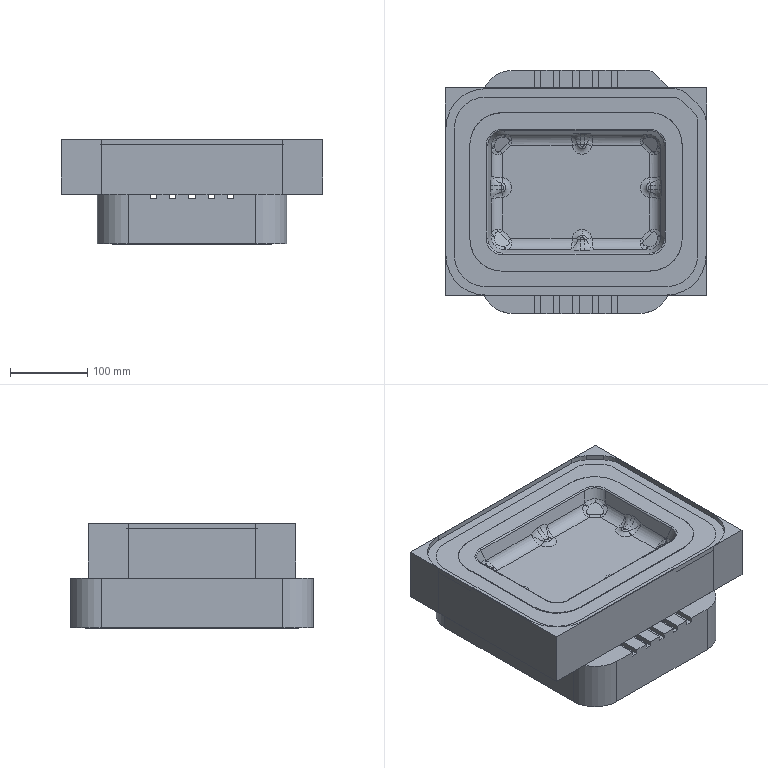NC program | NX | posted with a generic post | part box 339.125 x 315.125 x 135.5 mm
Lines 1 to 1308 of 120728:
N10 G17 G21 G94 G90
(B1 , TOOL : D16R0.8)
N12 T00 M6
N14 G53
N16 G17 G0 G90 X-27.429 Y125.5 S7000 M3 M8
N18 G43 Z220.5 H0
N20 Z71.5
N22 G94 G1 X0. Z70.063 F4500.
N24 X126.349
N26 G2 X138.946 Y120.282 R17.815
N28 G1 X155.159 Y104.069
N30 G2 X160.377 Y91.472 R17.815
N32 G1 Y-82.685
N34 G2 X117.563 Y-125.5 R42.815
N36 G1 X-117.563
N38 G2 X-160.377 Y-82.685 R42.815
N40 G1 Y82.685
N42 G2 X-117.563 Y125.5 R42.815
N44 G1 X0.
N46 Y115.42
N48 X126.349
N50 G2 X131.818 Y113.154 R7.735
N52 G1 X148.032 Y96.941
N54 G2 X150.297 Y91.472 R7.735
N56 G1 Y-82.685
N58 G2 X117.563 Y-115.42 R32.735
N60 G1 X-117.563
N62 G2 X-150.297 Y-82.685 R32.735
N64 G1 Y82.685
N66 G2 X-117.563 Y115.42 R32.735
N68 G1 X0.
N70 Y105.34
N72 X125.378
N74 X140.217 Y90.5
N76 Y-82.685
N78 G2 X117.563 Y-105.34 R22.655
N80 G1 X-117.563
N82 G2 X-140.217 Y-82.685 R22.655
N84 G1 Y82.685
N86 G2 X-117.563 Y105.34 R22.655
N88 G1 X0.
N90 Y95.26
N92 X121.203
N94 X130.137 Y86.325
N96 Y-82.685
N98 G2 X117.563 Y-95.26 R12.575
N100 G1 X-117.563
N102 G2 X-130.137 Y-82.685 R12.575
N104 G1 Y82.685
N106 G2 X-117.563 Y95.26 R12.575
N108 G1 X0.
N110 Y85.18
N112 X117.027
N114 X120.057 Y82.15
N116 Y-82.685
N118 G2 X117.563 Y-85.18 R2.495
N120 G1 X-117.563
N122 G2 X-120.057 Y-82.685 R2.495
N124 G1 Y82.685
N126 G2 X-117.563 Y85.18 R2.495
N128 G1 X0.
N130 Y75.1
N132 X109.977
N134 Y-75.1
N136 X-109.977
N138 Y75.1
N140 X0.
N142 Y65.02
N144 X99.897
N146 Y-65.02
N148 X-99.897
N150 Y65.02
N152 X0.
N154 Y54.94
N156 X89.817
N158 Y-54.94
N160 X-89.817
N162 Y54.94
N164 X0.
N166 Y44.86
N168 X79.737
N170 Y-44.86
N172 X-79.737
N174 Y44.86
N176 X0.
N178 Y34.78
N180 X69.657
N182 Y-34.78
N184 X-69.657
N186 Y34.78
N188 X0.
N190 Y24.7
N192 X59.577
N194 Y-24.7
N196 X-59.577
N198 Y24.7
N200 X0.
N202 Y14.62
N204 X49.497
N206 Y-14.62
N208 X-49.497
N210 Y14.62
N212 X0.
N214 Y4.54
N216 X39.417
N218 Y-4.54
N220 X-39.417
N222 Y4.54
N224 X0.
N226 G3 X3.2 Y7.74 R3.2
N228 G1 Z71.063
N230 G0 Z73.5
N232 X-27.429 Y125.435
N234 Z71.063
N236 G1 X0. Z69.625
N238 X126.349
N240 G2 X138.9 Y120.236 R17.75
N242 G1 X155.114 Y104.023
N244 G2 X160.313 Y91.472 R17.75
N246 G1 Y-82.685
N248 G2 X117.563 Y-125.435 R42.75
N250 G1 X-117.563
N252 G2 X-160.313 Y-82.685 R42.75
N254 G1 Y82.685
N256 G2 X-117.563 Y125.435 R42.75
N258 G1 X0.
N260 Y115.355
N262 X126.349
N264 G2 X131.773 Y113.109 R7.67
N266 G1 X147.986 Y96.895
N268 G2 X150.233 Y91.472 R7.67
N270 G1 Y-82.685
N272 G2 X117.563 Y-115.355 R32.67
N274 G1 X-117.563
N276 G2 X-150.233 Y-82.685 R32.67
N278 G1 Y82.685
N280 G2 X-117.563 Y115.355 R32.67
N282 G1 X0.
N284 Y105.275
N286 X125.351
N288 X140.153 Y90.474
N290 Y-82.686
N292 G2 X117.563 Y-105.275 R22.59
N294 G1 X-117.563
N296 G2 X-140.153 Y-82.685 R22.59
N298 G1 Y82.685
N300 G2 X-117.563 Y105.275 R22.59
N302 G1 X0.
N304 Y95.195
N306 X121.176
N308 X130.073 Y86.298
N310 Y-82.687
N312 G2 X117.563 Y-95.195 R12.51
N314 G1 X-117.563
N316 G2 X-130.073 Y-82.685 R12.51
N318 G1 Y82.685
N320 G2 X-117.563 Y95.195 R12.51
N322 G1 X0.
N324 Y85.115
N326 X117.
N328 X119.993 Y82.123
N330 Y-82.686
N332 G2 X117.563 Y-85.115 R2.43
N334 G1 X-117.563
N336 G2 X-119.993 Y-82.685 R2.43
N338 G1 Y82.685
N340 G2 X-117.563 Y85.115 R2.43
N342 G1 X0.
N344 Y75.035
N346 X109.913
N348 Y-75.035
N350 X-109.913
N352 Y75.035
N354 X0.
N356 Y64.955
N358 X99.833
N360 Y-64.955
N362 X-99.833
N364 Y64.955
N366 X0.
N368 Y54.875
N370 X89.753
N372 Y-54.875
N374 X-89.753
N376 Y54.875
N378 X0.
N380 Y44.795
N382 X79.673
N384 Y-44.795
N386 X-79.673
N388 Y44.795
N390 X0.
N392 Y34.715
N394 X69.593
N396 Y-34.715
N398 X-69.593
N400 Y34.715
N402 X0.
N404 Y24.635
N406 X59.513
N408 Y-24.635
N410 X-59.513
N412 Y24.635
N414 X0.
N416 Y14.555
N418 X49.433
N420 Y-14.555
N422 X-49.433
N424 Y14.555
N426 X0.
N428 Y4.475
N430 X39.353
N432 Y-4.475
N434 X-39.353
N436 Y4.475
N438 X0.
N440 G3 X3.2 Y7.675 R3.2
N442 G1 Z70.625
N444 G0 Z73.063
N446 X-27.429 Y125.435
N448 Z70.625
N450 G1 X0. Z69.188
N452 X126.349
N454 G2 X138.9 Y120.236 R17.75
N456 G1 X155.114 Y104.023
N458 G2 X160.313 Y91.472 R17.75
N460 G1 Y-82.685
N462 G2 X117.563 Y-125.435 R42.75
N464 G1 X-117.563
N466 G2 X-160.313 Y-82.685 R42.75
N468 G1 Y82.685
N470 G2 X-117.563 Y125.435 R42.75
N472 G1 X0.
N474 Y115.355
N476 X126.349
N478 G2 X131.773 Y113.109 R7.67
N480 G1 X147.986 Y96.895
N482 G2 X150.233 Y91.472 R7.67
N484 G1 Y-82.685
N486 G2 X117.563 Y-115.355 R32.67
N488 G1 X-117.563
N490 G2 X-150.233 Y-82.685 R32.67
N492 G1 Y82.685
N494 G2 X-117.563 Y115.355 R32.67
N496 G1 X0.
N498 Y105.275
N500 X125.351
N502 X140.153 Y90.474
N504 Y-82.686
N506 G2 X117.563 Y-105.275 R22.59
N508 G1 X-117.563
N510 G2 X-140.153 Y-82.685 R22.59
N512 G1 Y82.685
N514 G2 X-117.563 Y105.275 R22.59
N516 G1 X0.
N518 Y95.195
N520 X121.176
N522 X130.073 Y86.298
N524 Y-82.687
N526 G2 X117.563 Y-95.195 R12.51
N528 G1 X-117.563
N530 G2 X-130.073 Y-82.685 R12.51
N532 G1 Y82.685
N534 G2 X-117.563 Y95.195 R12.51
N536 G1 X0.
N538 Y85.115
N540 X117.
N542 X119.993 Y82.123
N544 Y-82.686
N546 G2 X117.563 Y-85.115 R2.43
N548 G1 X-117.563
N550 G2 X-119.993 Y-82.685 R2.43
N552 G1 Y82.685
N554 G2 X-117.563 Y85.115 R2.43
N556 G1 X0.
N558 Y75.035
N560 X109.913
N562 Y-75.035
N564 X-109.913
N566 Y75.035
N568 X0.
N570 Y64.955
N572 X99.833
N574 Y-64.955
N576 X-99.833
N578 Y64.955
N580 X0.
N582 Y54.875
N584 X89.753
N586 Y-54.875
N588 X-89.753
N590 Y54.875
N592 X0.
N594 Y44.795
N596 X79.673
N598 Y-44.795
N600 X-79.673
N602 Y44.795
N604 X0.
N606 Y34.715
N608 X69.593
N610 Y-34.715
N612 X-69.593
N614 Y34.715
N616 X0.
N618 Y24.635
N620 X59.513
N622 Y-24.635
N624 X-59.513
N626 Y24.635
N628 X0.
N630 Y14.555
N632 X49.433
N634 Y-14.555
N636 X-49.433
N638 Y14.555
N640 X0.
N642 Y4.475
N644 X39.353
N646 Y-4.475
N648 X-39.353
N650 Y4.475
N652 X0.
N654 G3 X3.2 Y7.675 R3.2
N656 G1 Z70.188
N658 G0 Z72.625
N660 X-27.429 Y125.435
N662 Z70.188
N664 G1 X0. Z68.75
N666 X126.349
N668 G2 X138.9 Y120.236 R17.75
N670 G1 X155.114 Y104.023
N672 G2 X160.313 Y91.472 R17.75
N674 G1 Y-82.685
N676 G2 X117.563 Y-125.435 R42.75
N678 G1 X-117.563
N680 G2 X-160.313 Y-82.685 R42.75
N682 G1 Y82.685
N684 G2 X-117.563 Y125.435 R42.75
N686 G1 X0.
N688 Y115.355
N690 X126.349
N692 G2 X131.773 Y113.109 R7.67
N694 G1 X147.986 Y96.895
N696 G2 X150.233 Y91.472 R7.67
N698 G1 Y-82.685
N700 G2 X117.563 Y-115.355 R32.67
N702 G1 X-117.563
N704 G2 X-150.233 Y-82.685 R32.67
N706 G1 Y82.685
N708 G2 X-117.563 Y115.355 R32.67
N710 G1 X0.
N712 Y105.275
N714 X125.351
N716 X140.153 Y90.474
N718 Y-82.686
N720 G2 X117.563 Y-105.275 R22.59
N722 G1 X-117.563
N724 G2 X-140.153 Y-82.685 R22.59
N726 G1 Y82.685
N728 G2 X-117.563 Y105.275 R22.59
N730 G1 X0.
N732 Y95.195
N734 X121.176
N736 X130.073 Y86.298
N738 Y-82.687
N740 G2 X117.563 Y-95.195 R12.51
N742 G1 X-117.563
N744 G2 X-130.073 Y-82.685 R12.51
N746 G1 Y82.685
N748 G2 X-117.563 Y95.195 R12.51
N750 G1 X0.
N752 Y85.115
N754 X117.
N756 X119.993 Y82.123
N758 Y-82.686
N760 G2 X117.563 Y-85.115 R2.43
N762 G1 X-117.563
N764 G2 X-119.993 Y-82.685 R2.43
N766 G1 Y82.685
N768 G2 X-117.563 Y85.115 R2.43
N770 G1 X0.
N772 Y75.035
N774 X109.913
N776 Y-75.035
N778 X-109.913
N780 Y75.035
N782 X0.
N784 Y64.955
N786 X99.833
N788 Y-64.955
N790 X-99.833
N792 Y64.955
N794 X0.
N796 Y54.875
N798 X89.753
N800 Y-54.875
N802 X-89.753
N804 Y54.875
N806 X0.
N808 Y44.795
N810 X79.673
N812 Y-44.795
N814 X-79.673
N816 Y44.795
N818 X0.
N820 Y34.715
N822 X69.593
N824 Y-34.715
N826 X-69.593
N828 Y34.715
N830 X0.
N832 Y24.635
N834 X59.513
N836 Y-24.635
N838 X-59.513
N840 Y24.635
N842 X0.
N844 Y14.555
N846 X49.433
N848 Y-14.555
N850 X-49.433
N852 Y14.555
N854 X0.
N856 Y4.475
N858 X39.353
N860 Y-4.475
N862 X-39.353
N864 Y4.475
N866 X0.
N868 G3 X3.2 Y7.675 R3.2
N870 G1 Z69.75
N872 G0 Z72.188
N874 X-27.429 Y125.435
N876 Z69.75
N878 G1 X0. Z68.313
N880 X126.349
N882 G2 X138.9 Y120.236 R17.75
N884 G1 X155.114 Y104.023
N886 G2 X160.313 Y91.472 R17.75
N888 G1 Y-82.685
N890 G2 X117.563 Y-125.435 R42.75
N892 G1 X-117.563
N894 G2 X-160.313 Y-82.685 R42.75
N896 G1 Y82.685
N898 G2 X-117.563 Y125.435 R42.75
N900 G1 X0.
N902 Y115.355
N904 X126.349
N906 G2 X131.773 Y113.109 R7.67
N908 G1 X147.986 Y96.895
N910 G2 X150.233 Y91.472 R7.67
N912 G1 Y-82.685
N914 G2 X117.563 Y-115.355 R32.67
N916 G1 X-117.563
N918 G2 X-150.233 Y-82.685 R32.67
N920 G1 Y82.685
N922 G2 X-117.563 Y115.355 R32.67
N924 G1 X0.
N926 Y105.275
N928 X125.351
N930 X140.153 Y90.474
N932 Y-82.686
N934 G2 X117.563 Y-105.275 R22.59
N936 G1 X-117.563
N938 G2 X-140.153 Y-82.685 R22.59
N940 G1 Y82.685
N942 G2 X-117.563 Y105.275 R22.59
N944 G1 X0.
N946 Y95.195
N948 X121.176
N950 X130.073 Y86.298
N952 Y-82.687
N954 G2 X117.563 Y-95.195 R12.51
N956 G1 X-117.563
N958 G2 X-130.073 Y-82.685 R12.51
N960 G1 Y82.685
N962 G2 X-117.563 Y95.195 R12.51
N964 G1 X0.
N966 Y85.115
N968 X117.
N970 X119.993 Y82.123
N972 Y-82.686
N974 G2 X117.563 Y-85.115 R2.43
N976 G1 X-117.563
N978 G2 X-119.993 Y-82.685 R2.43
N980 G1 Y82.685
N982 G2 X-117.563 Y85.115 R2.43
N984 G1 X0.
N986 Y75.035
N988 X109.913
N990 Y-75.035
N992 X-109.913
N994 Y75.035
N996 X0.
N998 Y64.955
N1000 X99.833
N1002 Y-64.955
N1004 X-99.833
N1006 Y64.955
N1008 X0.
N1010 Y54.875
N1012 X89.753
N1014 Y-54.875
N1016 X-89.753
N1018 Y54.875
N1020 X0.
N1022 Y44.795
N1024 X79.673
N1026 Y-44.795
N1028 X-79.673
N1030 Y44.795
N1032 X0.
N1034 Y34.715
N1036 X69.593
N1038 Y-34.715
N1040 X-69.593
N1042 Y34.715
N1044 X0.
N1046 Y24.635
N1048 X59.513
N1050 Y-24.635
N1052 X-59.513
N1054 Y24.635
N1056 X0.
N1058 Y14.555
N1060 X49.433
N1062 Y-14.555
N1064 X-49.433
N1066 Y14.555
N1068 X0.
N1070 Y4.475
N1072 X39.353
N1074 Y-4.475
N1076 X-39.353
N1078 Y4.475
N1080 X0.
N1082 G3 X3.2 Y7.675 R3.2
N1084 G1 Z69.313
N1086 G0 Z71.75
N1088 X-27.429 Y125.435
N1090 Z69.313
N1092 G1 X0. Z67.875
N1094 X126.349
N1096 G2 X138.9 Y120.236 R17.75
N1098 G1 X155.114 Y104.023
N1100 G2 X160.313 Y91.472 R17.75
N1102 G1 Y-82.685
N1104 G2 X117.563 Y-125.435 R42.75
N1106 G1 X-117.563
N1108 G2 X-160.313 Y-82.685 R42.75
N1110 G1 Y82.685
N1112 G2 X-117.563 Y125.435 R42.75
N1114 G1 X0.
N1116 Y115.355
N1118 X126.349
N1120 G2 X131.773 Y113.109 R7.67
N1122 G1 X147.986 Y96.895
N1124 G2 X150.233 Y91.472 R7.67
N1126 G1 Y-82.685
N1128 G2 X117.563 Y-115.355 R32.67
N1130 G1 X-117.563
N1132 G2 X-150.233 Y-82.685 R32.67
N1134 G1 Y82.685
N1136 G2 X-117.563 Y115.355 R32.67
N1138 G1 X0.
N1140 Y105.275
N1142 X125.351
N1144 X140.153 Y90.474
N1146 Y-82.686
N1148 G2 X117.563 Y-105.275 R22.59
N1150 G1 X-117.563
N1152 G2 X-140.153 Y-82.685 R22.59
N1154 G1 Y82.685
N1156 G2 X-117.563 Y105.275 R22.59
N1158 G1 X0.
N1160 Y95.195
N1162 X121.176
N1164 X130.073 Y86.298
N1166 Y-82.687
N1168 G2 X117.563 Y-95.195 R12.51
N1170 G1 X-117.563
N1172 G2 X-130.073 Y-82.685 R12.51
N1174 G1 Y82.685
N1176 G2 X-117.563 Y95.195 R12.51
N1178 G1 X0.
N1180 Y85.115
N1182 X117.
N1184 X119.993 Y82.123
N1186 Y-82.686
N1188 G2 X117.563 Y-85.115 R2.43
N1190 G1 X-117.563
N1192 G2 X-119.993 Y-82.685 R2.43
N1194 G1 Y82.685
N1196 G2 X-117.563 Y85.115 R2.43
N1198 G1 X0.
N1200 Y75.035
N1202 X109.913
N1204 Y-75.035
N1206 X-109.913
N1208 Y75.035
N1210 X0.
N1212 Y64.955
N1214 X99.833
N1216 Y-64.955
N1218 X-99.833
N1220 Y64.955
N1222 X0.
N1224 Y54.875
N1226 X89.753
N1228 Y-54.875
N1230 X-89.753
N1232 Y54.875
N1234 X0.
N1236 Y44.795
N1238 X79.673
N1240 Y-44.795
N1242 X-79.673
N1244 Y44.795
N1246 X0.
N1248 Y34.715
N1250 X69.593
N1252 Y-34.715
N1254 X-69.593
N1256 Y34.715
N1258 X0.
N1260 Y24.635
N1262 X59.513
N1264 Y-24.635
N1266 X-59.513
N1268 Y24.635
N1270 X0.
N1272 Y14.555
N1274 X49.433
N1276 Y-14.555
N1278 X-49.433
N1280 Y14.555
N1282 X0.
N1284 Y4.475
N1286 X39.353
N1288 Y-4.475
N1290 X-39.353
N1292 Y4.475
N1294 X0.
N1296 G3 X3.2 Y7.675 R3.2
N1298 G1 Z68.875
N1300 G0 Z71.313
N1302 X-27.429 Y125.435
N1304 Z68.875
N1306 G1 X0. Z67.438
N1308 X126.349
N1310 G2 X138.9 Y120.236 R17.75
N1312 G1 X155.114 Y104.023
N1314 G2 X160.313 Y91.472 R17.75
N1316 G1 Y-82.685
N1318 G2 X117.563 Y-125.435 R42.75
N1320 G1 X-117.563
N1322 G2 X-160.313 Y-82.685 R42.75
N1324 G1 Y82.685
N1326 G2 X-117.563 Y125.435 R42.75
N1328 G1 X0.
N1330 Y115.355
N1332 X126.349
N1334 G2 X131.773 Y113.109 R7.67
N1336 G1 X147.986 Y96.895
N1338 G2 X150.233 Y91.472 R7.67
N1340 G1 Y-82.685
N1342 G2 X117.563 Y-115.355 R32.67
N1344 G1 X-117.563
N1346 G2 X-150.233 Y-82.685 R32.67
N1348 G1 Y82.685
N1350 G2 X-117.563 Y115.355 R32.67
N1352 G1 X0.
N1354 Y105.275
N1356 X125.351
N1358 X140.153 Y90.474
N1360 Y-82.686
N1362 G2 X117.563 Y-105.275 R22.59
N1364 G1 X-117.563
N1366 G2 X-140.153 Y-82.685 R22.59
N1368 G1 Y82.685
N1370 G2 X-117.563 Y105.275 R22.59
N1372 G1 X0.
N1374 Y95.195
N1376 X121.176
N1378 X130.073 Y86.298
N1380 Y-82.687
N1382 G2 X117.563 Y-95.195 R12.51
N1384 G1 X-117.563
N1386 G2 X-130.073 Y-82.685 R12.51
N1388 G1 Y82.685
N1390 G2 X-117.563 Y95.195 R12.51
N1392 G1 X0.
N1394 Y85.115
N1396 X117.
N1398 X119.993 Y82.123
N1400 Y-82.686
N1402 G2 X117.563 Y-85.115 R2.43
N1404 G1 X-117.563
N1406 G2 X-119.993 Y-82.685 R2.43
N1408 G1 Y82.685
N1410 G2 X-117.563 Y85.115 R2.43
N1412 G1 X0.
N1414 Y75.035
N1416 X109.913
N1418 Y-75.035
N1420 X-109.913
N1422 Y75.035
N1424 X0.
N1426 Y64.955
N1428 X99.833
N1430 Y-64.955
N1432 X-99.833
N1434 Y64.955
N1436 X0.
N1438 Y54.875
N1440 X89.753
N1442 Y-54.875
N1444 X-89.753
N1446 Y54.875
N1448 X0.
N1450 Y44.795
N1452 X79.673
N1454 Y-44.795
N1456 X-79.673
N1458 Y44.795
N1460 X0.
N1462 Y34.715
N1464 X69.593
N1466 Y-34.715
N1468 X-69.593
N1470 Y34.715
N1472 X0.
N1474 Y24.635
N1476 X59.513
N1478 Y-24.635
N1480 X-59.513
N1482 Y24.635
N1484 X0.
N1486 Y14.555
N1488 X49.433
N1490 Y-14.555
N1492 X-49.433
N1494 Y14.555
N1496 X0.
N1498 Y4.475
N1500 X39.353
N1502 Y-4.475
N1504 X-39.353
N1506 Y4.475
N1508 X0.
N1510 G3 X3.2 Y7.675 R3.2
N1512 G1 Z68.438
N1514 G0 Z70.875
N1516 X-27.429 Y125.435
N1518 Z68.438
N1520 G1 X0. Z67.
N1522 X126.349
N1524 G2 X138.9 Y120.236 R17.75
N1526 G1 X155.114 Y104.023
N1528 G2 X160.313 Y91.472 R17.75
N1530 G1 Y-82.685
N1532 G2 X117.563 Y-125.435 R42.75
N1534 G1 X-117.563
N1536 G2 X-160.313 Y-82.685 R42.75
N1538 G1 Y82.685
N1540 G2 X-117.563 Y125.435 R42.75
N1542 G1 X0.
N1544 Y115.355
N1546 X126.349
N1548 G2 X131.773 Y113.109 R7.67
N1550 G1 X147.986 Y96.895
N1552 G2 X150.233 Y91.472 R7.67
N1554 G1 Y-82.685
N1556 G2 X117.563 Y-115.355 R32.67
N1558 G1 X-117.563
N1560 G2 X-150.233 Y-82.685 R32.67
N1562 G1 Y82.685
N1564 G2 X-117.563 Y115.355 R32.67
N1566 G1 X0.
N1568 Y105.275
N1570 X125.351
N1572 X140.153 Y90.474
N1574 Y-82.686
N1576 G2 X117.563 Y-105.275 R22.59
N1578 G1 X-117.563
N1580 G2 X-140.153 Y-82.685 R22.59
N1582 G1 Y82.685
N1584 G2 X-117.563 Y105.275 R22.59
N1586 G1 X0.
N1588 Y95.195
N1590 X121.176
N1592 X130.073 Y86.298
N1594 Y-82.687
N1596 G2 X117.563 Y-95.195 R12.51
N1598 G1 X-117.563
N1600 G2 X-130.073 Y-82.685 R12.51
N1602 G1 Y82.685
N1604 G2 X-117.563 Y95.195 R12.51
N1606 G1 X0.
N1608 Y85.115
N1610 X117.
N1612 X119.993 Y82.123
N1614 Y-82.686
N1616 G2 X117.563 Y-85.115 R2.43
N1618 G1 X-117.563
N1620 G2 X-119.993 Y-82.685 R2.43
N1622 G1 Y82.685
N1624 G2 X-117.563 Y85.115 R2.43
N1626 G1 X0.
N1628 Y75.035
N1630 X109.913
N1632 Y-75.035
N1634 X-109.913
N1636 Y75.035
N1638 X0.
N1640 Y64.955
N1642 X99.833
N1644 Y-64.955
N1646 X-99.833
N1648 Y64.955
N1650 X0.
N1652 Y54.875
N1654 X89.753
N1656 Y-54.875
N1658 X-89.753
N1660 Y54.875
N1662 X0.
N1664 Y44.795
N1666 X79.673
N1668 Y-44.795
N1670 X-79.673
N1672 Y44.795
N1674 X0.
N1676 Y34.715
N1678 X69.593
N1680 Y-34.715
N1682 X-69.593
N1684 Y34.715
N1686 X0.
N1688 Y24.635
N1690 X59.513
N1692 Y-24.635
N1694 X-59.513
N1696 Y24.635
N1698 X0.
N1700 Y14.555
N1702 X49.433
N1704 Y-14.555
N1706 X-49.433
N1708 Y14.555
N1710 X0.
N1712 Y4.475
N1714 X39.353
N1716 Y-4.475
N1718 X-39.353
N1720 Y4.475
N1722 X0.
N1724 G3 X3.2 Y7.675 R3.2
N1726 G1 Z68.
N1728 G0 Z70.438
N1730 X-27.429 Y125.435
N1732 Z68.
N1734 G1 X0. Z66.563
N1736 X126.349
N1738 G2 X138.9 Y120.236 R17.75
N1740 G1 X155.114 Y104.023
N1742 G2 X160.313 Y91.472 R17.75
N1744 G1 Y-82.685
N1746 G2 X117.563 Y-125.435 R42.75
N1748 G1 X-117.563
N1750 G2 X-160.313 Y-82.685 R42.75
N1752 G1 Y82.685
N1754 G2 X-117.563 Y125.435 R42.75
N1756 G1 X0.
N1758 Y115.355
N1760 X126.349
N1762 G2 X131.773 Y113.109 R7.67
N1764 G1 X147.986 Y96.895
N1766 G2 X150.233 Y91.472 R7.67
N1768 G1 Y-82.685
N1770 G2 X117.563 Y-115.355 R32.67
N1772 G1 X-117.563
N1774 G2 X-150.233 Y-82.685 R32.67
N1776 G1 Y82.685
N1778 G2 X-117.563 Y115.355 R32.67
N1780 G1 X0.
N1782 Y105.275
N1784 X125.351
N1786 X140.153 Y90.474
N1788 Y-82.686
N1790 G2 X117.563 Y-105.275 R22.59
N1792 G1 X-117.563
N1794 G2 X-140.153 Y-82.685 R22.59
N1796 G1 Y82.685
N1798 G2 X-117.563 Y105.275 R22.59
N1800 G1 X0.
N1802 Y95.195
N1804 X121.176
N1806 X130.073 Y86.298
N1808 Y-82.687
N1810 G2 X117.563 Y-95.195 R12.51
N1812 G1 X-117.563
N1814 G2 X-130.073 Y-82.685 R12.51
N1816 G1 Y82.685
N1818 G2 X-117.563 Y95.195 R12.51
N1820 G1 X0.
N1822 Y85.115
N1824 X117.
N1826 X119.993 Y82.123
N1828 Y-82.686
N1830 G2 X117.563 Y-85.115 R2.43
N1832 G1 X-117.563
N1834 G2 X-119.993 Y-82.685 R2.43
N1836 G1 Y82.685
N1838 G2 X-117.563 Y85.115 R2.43
N1840 G1 X0.
N1842 Y75.035
N1844 X109.913
N1846 Y-75.035
N1848 X-109.913
N1850 Y75.035
N1852 X0.
N1854 Y64.955
N1856 X99.833
N1858 Y-64.955
N1860 X-99.833
N1862 Y64.955
N1864 X0.
N1866 Y54.875
N1868 X89.753
N1870 Y-54.875
N1872 X-89.753
N1874 Y54.875
N1876 X0.
N1878 Y44.795
N1880 X79.673
N1882 Y-44.795
N1884 X-79.673
N1886 Y44.795
N1888 X0.
N1890 Y34.715
N1892 X69.593
N1894 Y-34.715
N1896 X-69.593
N1898 Y34.715
N1900 X0.
N1902 Y24.635
N1904 X59.513
N1906 Y-24.635
N1908 X-59.513
N1910 Y24.635
N1912 X0.
N1914 Y14.555
N1916 X49.433
N1918 Y-14.555
N1920 X-49.433
N1922 Y14.555
N1924 X0.
N1926 Y4.475
N1928 X39.353
N1930 Y-4.475
N1932 X-39.353
N1934 Y4.475
N1936 X0.
N1938 G3 X3.2 Y7.675 R3.2
N1940 G1 Z67.563
N1942 G0 Z70.
N1944 X-27.429 Y125.435
N1946 Z67.563
N1948 G1 X0. Z66.125
N1950 X126.349
N1952 G2 X138.9 Y120.236 R17.75
N1954 G1 X155.114 Y104.023
N1956 G2 X160.313 Y91.472 R17.75
N1958 G1 Y-82.685
N1960 G2 X117.563 Y-125.435 R42.75
N1962 G1 X-117.563
N1964 G2 X-160.313 Y-82.685 R42.75
N1966 G1 Y82.685
N1968 G2 X-117.563 Y125.435 R42.75
N1970 G1 X0.
N1972 Y115.355
N1974 X126.349
N1976 G2 X131.773 Y113.109 R7.67
N1978 G1 X147.986 Y96.895
N1980 G2 X150.233 Y91.472 R7.67
N1982 G1 Y-82.685
N1984 G2 X117.563 Y-115.355 R32.67
N1986 G1 X-117.563
N1988 G2 X-150.233 Y-82.685 R32.67
N1990 G1 Y82.685
N1992 G2 X-117.563 Y115.355 R32.67
N1994 G1 X0.
N1996 Y105.275
N1998 X125.351
N2000 X140.153 Y90.474
N2002 Y-82.686
N2004 G2 X117.563 Y-105.275 R22.59
N2006 G1 X-117.563
N2008 G2 X-140.153 Y-82.685 R22.59
N2010 G1 Y82.685
N2012 G2 X-117.563 Y105.275 R22.59
N2014 G1 X0.
N2016 Y95.195
N2018 X121.176
N2020 X130.073 Y86.298
N2022 Y-82.687
N2024 G2 X117.563 Y-95.195 R12.51
N2026 G1 X-117.563
N2028 G2 X-130.073 Y-82.685 R12.51
N2030 G1 Y82.685
N2032 G2 X-117.563 Y95.195 R12.51
N2034 G1 X0.
N2036 Y85.115
N2038 X117.
N2040 X119.993 Y82.123
N2042 Y-82.686
N2044 G2 X117.563 Y-85.115 R2.43
N2046 G1 X-117.563
N2048 G2 X-119.993 Y-82.685 R2.43
N2050 G1 Y82.685
N2052 G2 X-117.563 Y85.115 R2.43
N2054 G1 X0.
N2056 Y75.035
N2058 X109.913
N2060 Y-75.035
N2062 X-109.913
N2064 Y75.035
N2066 X0.
N2068 Y64.955
N2070 X99.833
N2072 Y-64.955
N2074 X-99.833
N2076 Y64.955
N2078 X0.
N2080 Y54.875
N2082 X89.753
N2084 Y-54.875
N2086 X-89.753
N2088 Y54.875
N2090 X0.
N2092 Y44.795
N2094 X79.673
N2096 Y-44.795
N2098 X-79.673
N2100 Y44.795
N2102 X0.
N2104 Y34.715
N2106 X69.593
N2108 Y-34.715
N2110 X-69.593
N2112 Y34.715
N2114 X0.
N2116 Y24.635
N2118 X59.513
N2120 Y-24.635
N2122 X-59.513
N2124 Y24.635
N2126 X0.
N2128 Y14.555
N2130 X49.433
N2132 Y-14.555
N2134 X-49.433
N2136 Y14.555
N2138 X0.
N2140 Y4.475
N2142 X39.353
N2144 Y-4.475
N2146 X-39.353
N2148 Y4.475
N2150 X0.
N2152 G3 X3.2 Y7.675 R3.2
N2154 G1 Z67.125
N2156 G0 Z69.563
N2158 X-27.429 Y125.435
N2160 Z67.125
N2162 G1 X0. Z65.688
N2164 X126.349
N2166 G2 X138.9 Y120.236 R17.75
N2168 G1 X155.114 Y104.023
N2170 G2 X160.313 Y91.472 R17.75
N2172 G1 Y-82.685
N2174 G2 X117.563 Y-125.435 R42.75
N2176 G1 X-117.563
N2178 G2 X-160.313 Y-82.685 R42.75
N2180 G1 Y82.685
N2182 G2 X-117.563 Y125.435 R42.75
N2184 G1 X0.
N2186 Y115.355
N2188 X126.349
N2190 G2 X131.773 Y113.109 R7.67
N2192 G1 X147.986 Y96.895
N2194 G2 X150.233 Y91.472 R7.67
N2196 G1 Y-82.685
N2198 G2 X117.563 Y-115.355 R32.67
N2200 G1 X-117.563
N2202 G2 X-150.233 Y-82.685 R32.67
N2204 G1 Y82.685
N2206 G2 X-117.563 Y115.355 R32.67
N2208 G1 X0.
N2210 Y105.275
N2212 X125.351
N2214 X140.153 Y90.474
N2216 Y-82.686
N2218 G2 X117.563 Y-105.275 R22.59
N2220 G1 X-117.563
N2222 G2 X-140.153 Y-82.685 R22.59
N2224 G1 Y82.685
N2226 G2 X-117.563 Y105.275 R22.59
N2228 G1 X0.
N2230 Y95.195
N2232 X121.176
N2234 X130.073 Y86.298
N2236 Y-82.687
N2238 G2 X117.563 Y-95.195 R12.51
N2240 G1 X-117.563
N2242 G2 X-130.073 Y-82.685 R12.51
N2244 G1 Y82.685
N2246 G2 X-117.563 Y95.195 R12.51
N2248 G1 X0.
N2250 Y85.115
N2252 X117.
N2254 X119.993 Y82.123
N2256 Y-82.686
N2258 G2 X117.563 Y-85.115 R2.43
N2260 G1 X-117.563
N2262 G2 X-119.993 Y-82.685 R2.43
N2264 G1 Y82.685
N2266 G2 X-117.563 Y85.115 R2.43
N2268 G1 X0.
N2270 Y75.035
N2272 X109.913
N2274 Y-75.035
N2276 X-109.913
N2278 Y75.035
N2280 X0.
N2282 Y64.955
N2284 X99.833
N2286 Y-64.955
N2288 X-99.833
N2290 Y64.955
N2292 X0.
N2294 Y54.875
N2296 X89.753
N2298 Y-54.875
N2300 X-89.753
N2302 Y54.875
N2304 X0.
N2306 Y44.795
N2308 X79.673
N2310 Y-44.795
N2312 X-79.673
N2314 Y44.795
N2316 X0.
N2318 Y34.715
N2320 X69.593
N2322 Y-34.715
N2324 X-69.593
N2326 Y34.715
N2328 X0.
N2330 Y24.635
N2332 X59.513
N2334 Y-24.635
N2336 X-59.513
N2338 Y24.635
N2340 X0.
N2342 Y14.555
N2344 X49.433
N2346 Y-14.555
N2348 X-49.433
N2350 Y14.555
N2352 X0.
N2354 Y4.475
N2356 X39.353
N2358 Y-4.475
N2360 X-39.353
N2362 Y4.475
N2364 X0.
N2366 G3 X3.2 Y7.675 R3.2
N2368 G1 Z66.688
N2370 G0 Z69.125
N2372 X-27.429 Y125.435
N2374 Z66.688
N2376 G1 X0. Z65.25
N2378 X126.349
N2380 G2 X138.9 Y120.236 R17.75
N2382 G1 X155.114 Y104.023
N2384 G2 X160.313 Y91.472 R17.75
N2386 G1 Y-82.685
N2388 G2 X117.563 Y-125.435 R42.75
N2390 G1 X-117.563
N2392 G2 X-160.313 Y-82.685 R42.75
N2394 G1 Y82.685
N2396 G2 X-117.563 Y125.435 R42.75
N2398 G1 X0.
N2400 Y115.355
N2402 X126.349
N2404 G2 X131.773 Y113.109 R7.67
N2406 G1 X147.986 Y96.895
N2408 G2 X150.233 Y91.472 R7.67
N2410 G1 Y-82.685
N2412 G2 X117.563 Y-115.355 R32.67
N2414 G1 X-117.563
N2416 G2 X-150.233 Y-82.685 R32.67
N2418 G1 Y82.685
N2420 G2 X-117.563 Y115.355 R32.67
N2422 G1 X0.
N2424 Y105.275
N2426 X125.351
N2428 X140.153 Y90.474
N2430 Y-82.686
N2432 G2 X117.563 Y-105.275 R22.59
N2434 G1 X-117.563
N2436 G2 X-140.153 Y-82.685 R22.59
N2438 G1 Y82.685
N2440 G2 X-117.563 Y105.275 R22.59
N2442 G1 X0.
N2444 Y95.195
N2446 X121.176
N2448 X130.073 Y86.298
N2450 Y-82.687
N2452 G2 X117.563 Y-95.195 R12.51
N2454 G1 X-117.563
N2456 G2 X-130.073 Y-82.685 R12.51
N2458 G1 Y82.685
N2460 G2 X-117.563 Y95.195 R12.51
N2462 G1 X0.
N2464 Y85.115
N2466 X117.
N2468 X119.993 Y82.123
N2470 Y-82.686
N2472 G2 X117.563 Y-85.115 R2.43
N2474 G1 X-117.563
N2476 G2 X-119.993 Y-82.685 R2.43
N2478 G1 Y82.685
N2480 G2 X-117.563 Y85.115 R2.43
N2482 G1 X0.
N2484 Y75.035
N2486 X109.913
N2488 Y-75.035
N2490 X-109.913
N2492 Y75.035
N2494 X0.
N2496 Y64.955
N2498 X99.833
N2500 Y-64.955
N2502 X-99.833
N2504 Y64.955
N2506 X0.
N2508 Y54.875
N2510 X89.753
N2512 Y-54.875
N2514 X-89.753
N2516 Y54.875
N2518 X0.
N2520 Y44.795
N2522 X79.673
N2524 Y-44.795
N2526 X-79.673
N2528 Y44.795
N2530 X0.
N2532 Y34.715
N2534 X69.593
N2536 Y-34.715
N2538 X-69.593
N2540 Y34.715
N2542 X0.
N2544 Y24.635
N2546 X59.513
N2548 Y-24.635
N2550 X-59.513
N2552 Y24.635
N2554 X0.
N2556 Y14.555
N2558 X49.433
N2560 Y-14.555
N2562 X-49.433
N2564 Y14.555
N2566 X0.
N2568 Y4.475
N2570 X39.353
N2572 Y-4.475
N2574 X-39.353
N2576 Y4.475
N2578 X0.
N2580 G3 X3.2 Y7.675 R3.2
N2582 G1 Z66.25
N2584 G0 Z68.688
N2586 X-25.441 Y72.852
N2588 Z66.25
N2590 G1 X0.001 Z64.917
N2592 X94.689
N2594 G2 X107.729 Y59.812 R12.783
N2596 G1 Y-59.812
N2598 G2 X94.689 Y-72.852 R12.782
N2600 G1 X-94.689
N2602 G2 X-107.729 Y-59.812 R12.783
N2604 G1 Y59.812
N2606 G2 X-94.689 Y72.852 R12.782
N2608 G1 X0.001
N2610 Y62.772
N2612 X94.792
N2614 G2 X97.649 Y59.914 R2.703